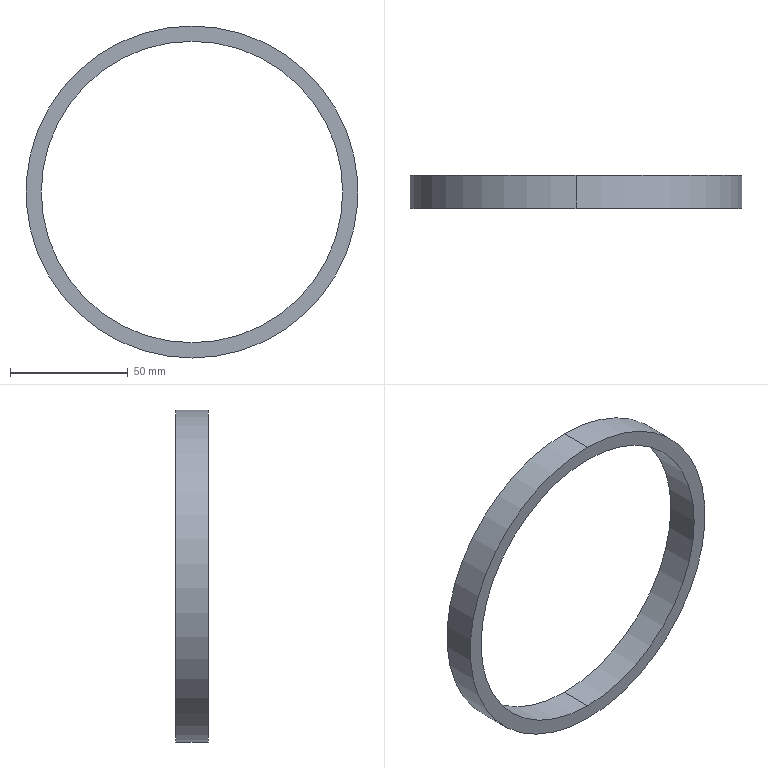Part | SolidWorks | features Revolution 1 | 1 solid | 6 faces | box 140.991 x 14 x 140.991 mm | volume 38449 mm3 | cylinder 4 | plane 2 | commonest cylinder face diameters 127.991 x2 140.991 x2
STEP:
#1=CARTESIAN_POINT('',(0.,137.5,-63.996));
#2=VERTEX_POINT('',#1);
#3=CARTESIAN_POINT('',(0.,137.5,63.996));
#4=VERTEX_POINT('',#3);
#5=CARTESIAN_POINT('',(0.,137.5,0.));
#6=DIRECTION('',(0.,1.,0.));
#7=DIRECTION('',(0.,0.,1.));
#8=AXIS2_PLACEMENT_3D('',#5,#6,#7);
#9=CIRCLE('',#8,63.996);
#10=EDGE_CURVE('',#2,#4,#9,.T.);
#11=ORIENTED_EDGE('',*,*,#10,.F.);
#12=CARTESIAN_POINT('',(0.,151.5,-63.996));
#13=VERTEX_POINT('',#12);
#14=CARTESIAN_POINT('',(0.,0.,-63.996));
#15=DIRECTION('',(0.,1.,0.));
#16=VECTOR('',#15,1000.);
#17=LINE('',#14,#16);
#18=EDGE_CURVE('',#2,#13,#17,.T.);
#19=ORIENTED_EDGE('',*,*,#18,.T.);
#20=CARTESIAN_POINT('',(0.,151.5,63.996));
#21=VERTEX_POINT('',#20);
#22=CARTESIAN_POINT('',(0.,151.5,0.));
#23=DIRECTION('',(0.,1.,0.));
#24=DIRECTION('',(0.,0.,1.));
#25=AXIS2_PLACEMENT_3D('',#22,#23,#24);
#26=CIRCLE('',#25,63.996);
#27=EDGE_CURVE('',#13,#21,#26,.T.);
#28=ORIENTED_EDGE('',*,*,#27,.T.);
#29=CARTESIAN_POINT('',(0.,0.,63.996));
#30=DIRECTION('',(0.,1.,0.));
#31=VECTOR('',#30,1000.);
#32=LINE('',#29,#31);
#33=EDGE_CURVE('',#4,#21,#32,.T.);
#34=ORIENTED_EDGE('',*,*,#33,.F.);
#35=EDGE_LOOP('',(#11,#19,#28,#34));
#36=FACE_OUTER_BOUND('',#35,.T.);
#37=CARTESIAN_POINT('',(0.,0.,0.));
#38=DIRECTION('',(0.,1.,0.));
#39=DIRECTION('',(0.,0.,1.));
#40=AXIS2_PLACEMENT_3D('',#37,#38,#39);
#41=CYLINDRICAL_SURFACE('',#40,63.996);
#42=ADVANCED_FACE('',(#36),#41,.F.);
#43=CARTESIAN_POINT('',(0.,137.5,70.496));
#44=VERTEX_POINT('',#43);
#45=CARTESIAN_POINT('',(0.,137.5,-70.496));
#46=VERTEX_POINT('',#45);
#47=CARTESIAN_POINT('',(0.,137.5,0.));
#48=DIRECTION('',(0.,1.,0.));
#49=DIRECTION('',(0.,0.,1.));
#50=AXIS2_PLACEMENT_3D('',#47,#48,#49);
#51=CIRCLE('',#50,70.496);
#52=EDGE_CURVE('',#44,#46,#51,.T.);
#53=ORIENTED_EDGE('',*,*,#52,.T.);
#54=CARTESIAN_POINT('',(0.,151.5,-70.496));
#55=VERTEX_POINT('',#54);
#56=CARTESIAN_POINT('',(0.,0.,-70.496));
#57=DIRECTION('',(0.,1.,0.));
#58=VECTOR('',#57,1000.);
#59=LINE('',#56,#58);
#60=EDGE_CURVE('',#46,#55,#59,.T.);
#61=ORIENTED_EDGE('',*,*,#60,.T.);
#62=CARTESIAN_POINT('',(0.,151.5,70.496));
#63=VERTEX_POINT('',#62);
#64=CARTESIAN_POINT('',(0.,151.5,0.));
#65=DIRECTION('',(0.,1.,0.));
#66=DIRECTION('',(0.,0.,1.));
#67=AXIS2_PLACEMENT_3D('',#64,#65,#66);
#68=CIRCLE('',#67,70.496);
#69=EDGE_CURVE('',#63,#55,#68,.T.);
#70=ORIENTED_EDGE('',*,*,#69,.F.);
#71=CARTESIAN_POINT('',(0.,0.,70.496));
#72=DIRECTION('',(0.,1.,0.));
#73=VECTOR('',#72,1000.);
#74=LINE('',#71,#73);
#75=EDGE_CURVE('',#44,#63,#74,.T.);
#76=ORIENTED_EDGE('',*,*,#75,.F.);
#77=EDGE_LOOP('',(#53,#61,#70,#76));
#78=FACE_OUTER_BOUND('',#77,.T.);
#79=CARTESIAN_POINT('',(0.,0.,0.));
#80=DIRECTION('',(0.,1.,0.));
#81=DIRECTION('',(0.,0.,1.));
#82=AXIS2_PLACEMENT_3D('',#79,#80,#81);
#83=CYLINDRICAL_SURFACE('',#82,70.496);
#84=ADVANCED_FACE('',(#78),#83,.T.);
#85=ORIENTED_EDGE('',*,*,#60,.F.);
#86=CARTESIAN_POINT('',(0.,137.5,0.));
#87=DIRECTION('',(0.,1.,0.));
#88=DIRECTION('',(0.,0.,1.));
#89=AXIS2_PLACEMENT_3D('',#86,#87,#88);
#90=CIRCLE('',#89,70.496);
#91=EDGE_CURVE('',#46,#44,#90,.T.);
#92=ORIENTED_EDGE('',*,*,#91,.T.);
#93=ORIENTED_EDGE('',*,*,#75,.T.);
#94=CARTESIAN_POINT('',(0.,151.5,0.));
#95=DIRECTION('',(0.,1.,0.));
#96=DIRECTION('',(0.,0.,1.));
#97=AXIS2_PLACEMENT_3D('',#94,#95,#96);
#98=CIRCLE('',#97,70.496);
#99=EDGE_CURVE('',#55,#63,#98,.T.);
#100=ORIENTED_EDGE('',*,*,#99,.F.);
#101=EDGE_LOOP('',(#85,#92,#93,#100));
#102=FACE_OUTER_BOUND('',#101,.T.);
#103=CARTESIAN_POINT('',(0.,0.,0.));
#104=DIRECTION('',(0.,1.,0.));
#105=DIRECTION('',(0.,0.,1.));
#106=AXIS2_PLACEMENT_3D('',#103,#104,#105);
#107=CYLINDRICAL_SURFACE('',#106,70.496);
#108=ADVANCED_FACE('',(#102),#107,.T.);
#109=ORIENTED_EDGE('',*,*,#52,.F.);
#110=ORIENTED_EDGE('',*,*,#91,.F.);
#111=EDGE_LOOP('',(#109,#110));
#112=FACE_OUTER_BOUND('',#111,.T.);
#113=CARTESIAN_POINT('',(0.,137.5,0.));
#114=DIRECTION('',(0.,1.,0.));
#115=DIRECTION('',(0.,0.,1.));
#116=AXIS2_PLACEMENT_3D('',#113,#114,#115);
#117=CIRCLE('',#116,63.996);
#118=EDGE_CURVE('',#4,#2,#117,.T.);
#119=ORIENTED_EDGE('',*,*,#118,.T.);
#120=ORIENTED_EDGE('',*,*,#10,.T.);
#121=EDGE_LOOP('',(#119,#120));
#122=FACE_BOUND('',#121,.T.);
#123=CARTESIAN_POINT('',(70.496,137.5,0.));
#124=DIRECTION('',(0.,1.,0.));
#125=DIRECTION('',(0.,0.,1.));
#126=AXIS2_PLACEMENT_3D('',#123,#124,#125);
#127=PLANE('',#126);
#128=ADVANCED_FACE('',(#112,#122),#127,.F.);
#129=ORIENTED_EDGE('',*,*,#18,.F.);
#130=ORIENTED_EDGE('',*,*,#118,.F.);
#131=ORIENTED_EDGE('',*,*,#33,.T.);
#132=CARTESIAN_POINT('',(0.,151.5,0.));
#133=DIRECTION('',(0.,1.,0.));
#134=DIRECTION('',(0.,0.,1.));
#135=AXIS2_PLACEMENT_3D('',#132,#133,#134);
#136=CIRCLE('',#135,63.996);
#137=EDGE_CURVE('',#21,#13,#136,.T.);
#138=ORIENTED_EDGE('',*,*,#137,.T.);
#139=EDGE_LOOP('',(#129,#130,#131,#138));
#140=FACE_OUTER_BOUND('',#139,.T.);
#141=CARTESIAN_POINT('',(0.,0.,0.));
#142=DIRECTION('',(0.,1.,0.));
#143=DIRECTION('',(0.,0.,1.));
#144=AXIS2_PLACEMENT_3D('',#141,#142,#143);
#145=CYLINDRICAL_SURFACE('',#144,63.996);
#146=ADVANCED_FACE('',(#140),#145,.F.);
#147=ORIENTED_EDGE('',*,*,#137,.F.);
#148=ORIENTED_EDGE('',*,*,#27,.F.);
#149=EDGE_LOOP('',(#147,#148));
#150=FACE_BOUND('',#149,.T.);
#151=ORIENTED_EDGE('',*,*,#69,.T.);
#152=ORIENTED_EDGE('',*,*,#99,.T.);
#153=EDGE_LOOP('',(#151,#152));
#154=FACE_OUTER_BOUND('',#153,.T.);
#155=CARTESIAN_POINT('',(70.496,151.5,0.));
#156=DIRECTION('',(0.,-1.,0.));
#157=DIRECTION('',(0.,0.,-1.));
#158=AXIS2_PLACEMENT_3D('',#155,#156,#157);
#159=PLANE('',#158);
#160=ADVANCED_FACE('',(#150,#154),#159,.F.);
#161=CLOSED_SHELL('',(#42,#84,#108,#128,#146,#160));
#162=MANIFOLD_SOLID_BREP('',#161);
#163=CARTESIAN_POINT('',(0.,0.,0.));
#164=DIRECTION('',(0.,0.,1.));
#165=DIRECTION('',(1.,0.,0.));
#166=AXIS2_PLACEMENT_3D('',#163,#164,#165);
#167=(LENGTH_UNIT()NAMED_UNIT(*)SI_UNIT(.MILLI.,.METRE.));
#168=UNCERTAINTY_MEASURE_WITH_UNIT(LENGTH_MEASURE(0.00001),#167,'','');
#169=(NAMED_UNIT(*)PLANE_ANGLE_UNIT()SI_UNIT($,.RADIAN.));
#170=(NAMED_UNIT(*)SI_UNIT($,.STERADIAN.)SOLID_ANGLE_UNIT());
#171=(GEOMETRIC_REPRESENTATION_CONTEXT(3)GLOBAL_UNCERTAINTY_ASSIGNED_CONTEXT((#168))GLOBAL_UNIT_ASSIGNED_CONTEXT((#167,#169,#170))REPRESENTATION_CONTEXT('',''));
#172=ADVANCED_BREP_SHAPE_REPRESENTATION('',(#162,#166),#171);